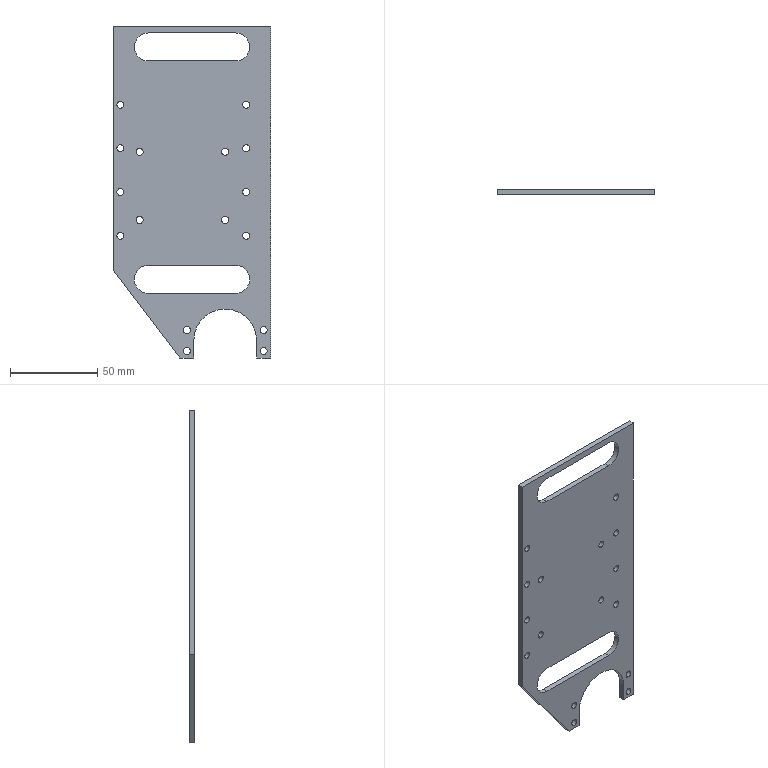Part | SolidWorks | features Extrusion 1, ICE 1 | 1 solid | 52 faces | box 90 x 3 x 190 mm | volume 39234 mm3 | cylinder 38 | plane 14 | commonest cylinder face diameters 4 x32 16 x4 36 x2